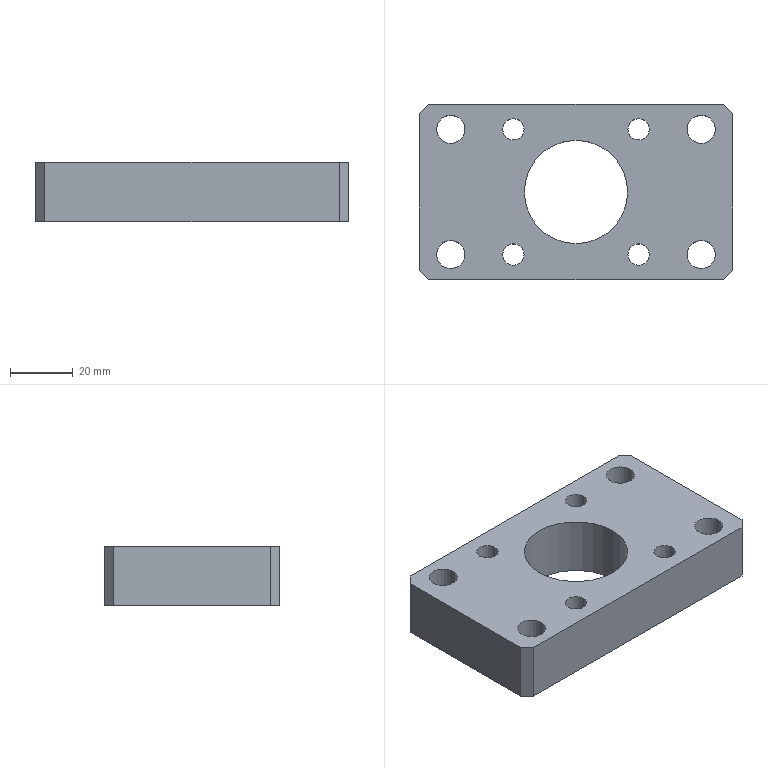Part | STEP file | Locking Cylinder Mounting Plate | 1 solid | 40 faces | box 100 x 56 x 19 mm | volume 79159 mm3 | cylinder 26 | plane 14 | commonest cylinder face diameters 6.8 x8 9 x8 11 x8 33 x2